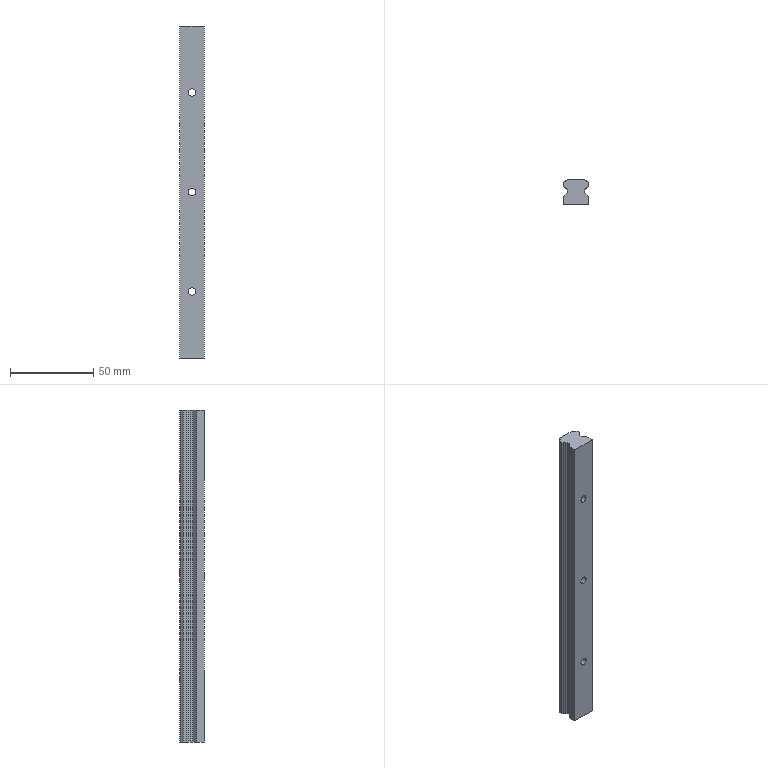Part | SolidWorks | features ICE 15, Chamfer 3, Extrusion 3, Fillet 3, MirrorPattern 3, MirrorSolid 3, RevCut 2, DeleteBody 1, Dome 1, LPattern 1 | 1 solid | 41 faces | box 15 x 15 x 200 mm | volume 39273 mm3 | plane 23 | cylinder 18 | commonest cylinder face diameters 1.459 x6 4.5 x6 7.5 x6
STEP:
#1=CARTESIAN_POINT('',(0.,5.3,-57.75));
#2=VERTEX_POINT('',#1);
#3=CARTESIAN_POINT('',(0.,5.3,-62.25));
#4=VERTEX_POINT('',#3);
#5=CARTESIAN_POINT('',(0.,5.3,-60.));
#6=DIRECTION('',(0.,-1.,0.));
#7=DIRECTION('',(0.,0.,-1.));
#8=AXIS2_PLACEMENT_3D('',#5,#6,#7);
#9=CIRCLE('',#8,2.25);
#10=EDGE_CURVE('',#2,#4,#9,.T.);
#11=ORIENTED_EDGE('',*,*,#10,.F.);
#12=CARTESIAN_POINT('',(0.,-4.4,-57.75));
#13=VERTEX_POINT('',#12);
#14=CARTESIAN_POINT('',(0.,-4.4,-57.75));
#15=DIRECTION('',(0.,-1.,0.));
#16=VECTOR('',#15,1000.);
#17=LINE('',#14,#16);
#18=EDGE_CURVE('',#2,#13,#17,.T.);
#19=ORIENTED_EDGE('',*,*,#18,.T.);
#20=CARTESIAN_POINT('',(0.,-4.4,-62.25));
#21=VERTEX_POINT('',#20);
#22=CARTESIAN_POINT('',(0.,-4.4,-60.));
#23=DIRECTION('',(0.,-1.,0.));
#24=DIRECTION('',(0.,0.,-1.));
#25=AXIS2_PLACEMENT_3D('',#22,#23,#24);
#26=CIRCLE('',#25,2.25);
#27=EDGE_CURVE('',#13,#21,#26,.T.);
#28=ORIENTED_EDGE('',*,*,#27,.T.);
#29=CARTESIAN_POINT('',(0.,-4.4,-62.25));
#30=DIRECTION('',(0.,-1.,0.));
#31=VECTOR('',#30,1000.);
#32=LINE('',#29,#31);
#33=EDGE_CURVE('',#4,#21,#32,.T.);
#34=ORIENTED_EDGE('',*,*,#33,.F.);
#35=EDGE_LOOP('',(#11,#19,#28,#34));
#36=FACE_OUTER_BOUND('',#35,.T.);
#37=CARTESIAN_POINT('',(0.,-4.4,-60.));
#38=DIRECTION('',(0.,-1.,0.));
#39=DIRECTION('',(0.,0.,-1.));
#40=AXIS2_PLACEMENT_3D('',#37,#38,#39);
#41=CYLINDRICAL_SURFACE('',#40,2.25);
#42=ADVANCED_FACE('',(#36),#41,.F.);
#43=CARTESIAN_POINT('',(0.,10.6,-56.25));
#44=VERTEX_POINT('',#43);
#45=CARTESIAN_POINT('',(0.,10.6,-63.75));
#46=VERTEX_POINT('',#45);
#47=CARTESIAN_POINT('',(0.,10.6,-60.));
#48=DIRECTION('',(0.,-1.,0.));
#49=DIRECTION('',(0.,0.,-1.));
#50=AXIS2_PLACEMENT_3D('',#47,#48,#49);
#51=CIRCLE('',#50,3.75);
#52=EDGE_CURVE('',#44,#46,#51,.T.);
#53=ORIENTED_EDGE('',*,*,#52,.F.);
#54=CARTESIAN_POINT('',(0.,5.3,-56.25));
#55=VERTEX_POINT('',#54);
#56=CARTESIAN_POINT('',(0.,-4.4,-56.25));
#57=DIRECTION('',(0.,-1.,0.));
#58=VECTOR('',#57,1000.);
#59=LINE('',#56,#58);
#60=EDGE_CURVE('',#44,#55,#59,.T.);
#61=ORIENTED_EDGE('',*,*,#60,.T.);
#62=CARTESIAN_POINT('',(0.,5.3,-63.75));
#63=VERTEX_POINT('',#62);
#64=CARTESIAN_POINT('',(0.,5.3,-60.));
#65=DIRECTION('',(0.,-1.,0.));
#66=DIRECTION('',(0.,0.,-1.));
#67=AXIS2_PLACEMENT_3D('',#64,#65,#66);
#68=CIRCLE('',#67,3.75);
#69=EDGE_CURVE('',#55,#63,#68,.T.);
#70=ORIENTED_EDGE('',*,*,#69,.T.);
#71=CARTESIAN_POINT('',(0.,-4.4,-63.75));
#72=DIRECTION('',(0.,-1.,0.));
#73=VECTOR('',#72,1000.);
#74=LINE('',#71,#73);
#75=EDGE_CURVE('',#46,#63,#74,.T.);
#76=ORIENTED_EDGE('',*,*,#75,.F.);
#77=EDGE_LOOP('',(#53,#61,#70,#76));
#78=FACE_OUTER_BOUND('',#77,.T.);
#79=CARTESIAN_POINT('',(0.,-4.4,-60.));
#80=DIRECTION('',(0.,-1.,0.));
#81=DIRECTION('',(0.,0.,-1.));
#82=AXIS2_PLACEMENT_3D('',#79,#80,#81);
#83=CYLINDRICAL_SURFACE('',#82,3.75);
#84=ADVANCED_FACE('',(#78),#83,.F.);
#85=CARTESIAN_POINT('',(0.,5.3,2.25));
#86=VERTEX_POINT('',#85);
#87=CARTESIAN_POINT('',(0.,5.3,-2.25));
#88=VERTEX_POINT('',#87);
#89=CARTESIAN_POINT('',(0.,5.3,0.));
#90=DIRECTION('',(0.,-1.,0.));
#91=DIRECTION('',(0.,0.,-1.));
#92=AXIS2_PLACEMENT_3D('',#89,#90,#91);
#93=CIRCLE('',#92,2.25);
#94=EDGE_CURVE('',#86,#88,#93,.T.);
#95=ORIENTED_EDGE('',*,*,#94,.F.);
#96=CARTESIAN_POINT('',(0.,-4.4,2.25));
#97=VERTEX_POINT('',#96);
#98=CARTESIAN_POINT('',(0.,-4.4,2.25));
#99=DIRECTION('',(0.,-1.,0.));
#100=VECTOR('',#99,1000.);
#101=LINE('',#98,#100);
#102=EDGE_CURVE('',#86,#97,#101,.T.);
#103=ORIENTED_EDGE('',*,*,#102,.T.);
#104=CARTESIAN_POINT('',(0.,-4.4,-2.25));
#105=VERTEX_POINT('',#104);
#106=CARTESIAN_POINT('',(0.,-4.4,0.));
#107=DIRECTION('',(0.,-1.,0.));
#108=DIRECTION('',(0.,0.,-1.));
#109=AXIS2_PLACEMENT_3D('',#106,#107,#108);
#110=CIRCLE('',#109,2.25);
#111=EDGE_CURVE('',#97,#105,#110,.T.);
#112=ORIENTED_EDGE('',*,*,#111,.T.);
#113=CARTESIAN_POINT('',(0.,-4.4,-2.25));
#114=DIRECTION('',(0.,-1.,0.));
#115=VECTOR('',#114,1000.);
#116=LINE('',#113,#115);
#117=EDGE_CURVE('',#88,#105,#116,.T.);
#118=ORIENTED_EDGE('',*,*,#117,.F.);
#119=EDGE_LOOP('',(#95,#103,#112,#118));
#120=FACE_OUTER_BOUND('',#119,.T.);
#121=CARTESIAN_POINT('',(0.,-4.4,0.));
#122=DIRECTION('',(0.,-1.,0.));
#123=DIRECTION('',(0.,0.,-1.));
#124=AXIS2_PLACEMENT_3D('',#121,#122,#123);
#125=CYLINDRICAL_SURFACE('',#124,2.25);
#126=ADVANCED_FACE('',(#120),#125,.F.);
#127=CARTESIAN_POINT('',(0.,10.6,3.75));
#128=VERTEX_POINT('',#127);
#129=CARTESIAN_POINT('',(0.,10.6,-3.75));
#130=VERTEX_POINT('',#129);
#131=CARTESIAN_POINT('',(0.,10.6,0.));
#132=DIRECTION('',(0.,-1.,0.));
#133=DIRECTION('',(0.,0.,-1.));
#134=AXIS2_PLACEMENT_3D('',#131,#132,#133);
#135=CIRCLE('',#134,3.75);
#136=EDGE_CURVE('',#128,#130,#135,.T.);
#137=ORIENTED_EDGE('',*,*,#136,.F.);
#138=CARTESIAN_POINT('',(0.,5.3,3.75));
#139=VERTEX_POINT('',#138);
#140=CARTESIAN_POINT('',(0.,-4.4,3.75));
#141=DIRECTION('',(0.,-1.,0.));
#142=VECTOR('',#141,1000.);
#143=LINE('',#140,#142);
#144=EDGE_CURVE('',#128,#139,#143,.T.);
#145=ORIENTED_EDGE('',*,*,#144,.T.);
#146=CARTESIAN_POINT('',(0.,5.3,-3.75));
#147=VERTEX_POINT('',#146);
#148=CARTESIAN_POINT('',(0.,5.3,0.));
#149=DIRECTION('',(0.,-1.,0.));
#150=DIRECTION('',(0.,0.,-1.));
#151=AXIS2_PLACEMENT_3D('',#148,#149,#150);
#152=CIRCLE('',#151,3.75);
#153=EDGE_CURVE('',#139,#147,#152,.T.);
#154=ORIENTED_EDGE('',*,*,#153,.T.);
#155=CARTESIAN_POINT('',(0.,-4.4,-3.75));
#156=DIRECTION('',(0.,-1.,0.));
#157=VECTOR('',#156,1000.);
#158=LINE('',#155,#157);
#159=EDGE_CURVE('',#130,#147,#158,.T.);
#160=ORIENTED_EDGE('',*,*,#159,.F.);
#161=EDGE_LOOP('',(#137,#145,#154,#160));
#162=FACE_OUTER_BOUND('',#161,.T.);
#163=CARTESIAN_POINT('',(0.,-4.4,0.));
#164=DIRECTION('',(0.,-1.,0.));
#165=DIRECTION('',(0.,0.,-1.));
#166=AXIS2_PLACEMENT_3D('',#163,#164,#165);
#167=CYLINDRICAL_SURFACE('',#166,3.75);
#168=ADVANCED_FACE('',(#162),#167,.F.);
#169=CARTESIAN_POINT('',(0.,5.3,62.25));
#170=VERTEX_POINT('',#169);
#171=CARTESIAN_POINT('',(0.,5.3,57.75));
#172=VERTEX_POINT('',#171);
#173=CARTESIAN_POINT('',(0.,5.3,60.));
#174=DIRECTION('',(0.,-1.,0.));
#175=DIRECTION('',(0.,0.,-1.));
#176=AXIS2_PLACEMENT_3D('',#173,#174,#175);
#177=CIRCLE('',#176,2.25);
#178=EDGE_CURVE('',#170,#172,#177,.T.);
#179=ORIENTED_EDGE('',*,*,#178,.F.);
#180=CARTESIAN_POINT('',(0.,-4.4,62.25));
#181=VERTEX_POINT('',#180);
#182=CARTESIAN_POINT('',(0.,-4.4,62.25));
#183=DIRECTION('',(0.,-1.,0.));
#184=VECTOR('',#183,1000.);
#185=LINE('',#182,#184);
#186=EDGE_CURVE('',#170,#181,#185,.T.);
#187=ORIENTED_EDGE('',*,*,#186,.T.);
#188=CARTESIAN_POINT('',(0.,-4.4,57.75));
#189=VERTEX_POINT('',#188);
#190=CARTESIAN_POINT('',(0.,-4.4,60.));
#191=DIRECTION('',(0.,-1.,0.));
#192=DIRECTION('',(0.,0.,-1.));
#193=AXIS2_PLACEMENT_3D('',#190,#191,#192);
#194=CIRCLE('',#193,2.25);
#195=EDGE_CURVE('',#181,#189,#194,.T.);
#196=ORIENTED_EDGE('',*,*,#195,.T.);
#197=CARTESIAN_POINT('',(0.,-4.4,57.75));
#198=DIRECTION('',(0.,-1.,0.));
#199=VECTOR('',#198,1000.);
#200=LINE('',#197,#199);
#201=EDGE_CURVE('',#172,#189,#200,.T.);
#202=ORIENTED_EDGE('',*,*,#201,.F.);
#203=EDGE_LOOP('',(#179,#187,#196,#202));
#204=FACE_OUTER_BOUND('',#203,.T.);
#205=CARTESIAN_POINT('',(0.,-4.4,60.));
#206=DIRECTION('',(0.,-1.,0.));
#207=DIRECTION('',(0.,0.,-1.));
#208=AXIS2_PLACEMENT_3D('',#205,#206,#207);
#209=CYLINDRICAL_SURFACE('',#208,2.25);
#210=ADVANCED_FACE('',(#204),#209,.F.);
#211=CARTESIAN_POINT('',(0.,10.6,63.75));
#212=VERTEX_POINT('',#211);
#213=CARTESIAN_POINT('',(0.,10.6,56.25));
#214=VERTEX_POINT('',#213);
#215=CARTESIAN_POINT('',(0.,10.6,60.));
#216=DIRECTION('',(0.,-1.,0.));
#217=DIRECTION('',(0.,0.,-1.));
#218=AXIS2_PLACEMENT_3D('',#215,#216,#217);
#219=CIRCLE('',#218,3.75);
#220=EDGE_CURVE('',#212,#214,#219,.T.);
#221=ORIENTED_EDGE('',*,*,#220,.F.);
#222=CARTESIAN_POINT('',(0.,5.3,63.75));
#223=VERTEX_POINT('',#222);
#224=CARTESIAN_POINT('',(0.,-4.4,63.75));
#225=DIRECTION('',(0.,-1.,0.));
#226=VECTOR('',#225,1000.);
#227=LINE('',#224,#226);
#228=EDGE_CURVE('',#212,#223,#227,.T.);
#229=ORIENTED_EDGE('',*,*,#228,.T.);
#230=CARTESIAN_POINT('',(0.,5.3,56.25));
#231=VERTEX_POINT('',#230);
#232=CARTESIAN_POINT('',(0.,5.3,60.));
#233=DIRECTION('',(0.,-1.,0.));
#234=DIRECTION('',(0.,0.,-1.));
#235=AXIS2_PLACEMENT_3D('',#232,#233,#234);
#236=CIRCLE('',#235,3.75);
#237=EDGE_CURVE('',#223,#231,#236,.T.);
#238=ORIENTED_EDGE('',*,*,#237,.T.);
#239=CARTESIAN_POINT('',(0.,-4.4,56.25));
#240=DIRECTION('',(0.,-1.,0.));
#241=VECTOR('',#240,1000.);
#242=LINE('',#239,#241);
#243=EDGE_CURVE('',#214,#231,#242,.T.);
#244=ORIENTED_EDGE('',*,*,#243,.F.);
#245=EDGE_LOOP('',(#221,#229,#238,#244));
#246=FACE_OUTER_BOUND('',#245,.T.);
#247=CARTESIAN_POINT('',(0.,-4.4,60.));
#248=DIRECTION('',(0.,-1.,0.));
#249=DIRECTION('',(0.,0.,-1.));
#250=AXIS2_PLACEMENT_3D('',#247,#248,#249);
#251=CYLINDRICAL_SURFACE('',#250,3.75);
#252=ADVANCED_FACE('',(#246),#251,.F.);
#253=CARTESIAN_POINT('',(-6.016,9.858,-100.));
#254=VERTEX_POINT('',#253);
#255=CARTESIAN_POINT('',(-6.016,9.846,-100.));
#256=VERTEX_POINT('',#255);
#257=CARTESIAN_POINT('',(-6.746,9.846,-100.));
#258=DIRECTION('',(0.,0.,-1.));
#259=DIRECTION('',(1.,0.,0.));
#260=AXIS2_PLACEMENT_3D('',#257,#258,#259);
#261=CIRCLE('',#260,0.7296);
#262=EDGE_CURVE('',#254,#256,#261,.T.);
#263=ORIENTED_EDGE('',*,*,#262,.T.);
#264=CARTESIAN_POINT('',(-6.016,9.846,100.));
#265=VERTEX_POINT('',#264);
#266=CARTESIAN_POINT('',(-6.016,9.846,-100.));
#267=DIRECTION('',(0.,0.,1.));
#268=VECTOR('',#267,1000.);
#269=LINE('',#266,#268);
#270=EDGE_CURVE('',#256,#265,#269,.T.);
#271=ORIENTED_EDGE('',*,*,#270,.T.);
#272=CARTESIAN_POINT('',(-6.016,9.858,100.));
#273=VERTEX_POINT('',#272);
#274=CARTESIAN_POINT('',(-6.746,9.846,100.));
#275=DIRECTION('',(0.,0.,-1.));
#276=DIRECTION('',(1.,0.,0.));
#277=AXIS2_PLACEMENT_3D('',#274,#275,#276);
#278=CIRCLE('',#277,0.7296);
#279=EDGE_CURVE('',#273,#265,#278,.T.);
#280=ORIENTED_EDGE('',*,*,#279,.F.);
#281=CARTESIAN_POINT('',(-6.016,9.858,-100.));
#282=DIRECTION('',(0.,0.,1.));
#283=VECTOR('',#282,1000.);
#284=LINE('',#281,#283);
#285=EDGE_CURVE('',#254,#273,#284,.T.);
#286=ORIENTED_EDGE('',*,*,#285,.F.);
#287=EDGE_LOOP('',(#263,#271,#280,#286));
#288=FACE_OUTER_BOUND('',#287,.T.);
#289=CARTESIAN_POINT('',(-6.746,9.846,-100.));
#290=DIRECTION('',(0.,0.,1.));
#291=DIRECTION('',(1.,0.,0.));
#292=AXIS2_PLACEMENT_3D('',#289,#290,#291);
#293=CYLINDRICAL_SURFACE('',#292,0.7296);
#294=ADVANCED_FACE('',(#288),#293,.F.);
#295=CARTESIAN_POINT('',(-6.758,5.724,-100.));
#296=VERTEX_POINT('',#295);
#297=CARTESIAN_POINT('',(-6.016,4.994,-100.));
#298=VERTEX_POINT('',#297);
#299=CARTESIAN_POINT('',(-6.746,4.994,-100.));
#300=DIRECTION('',(0.,0.,-1.));
#301=DIRECTION('',(1.,0.,0.));
#302=AXIS2_PLACEMENT_3D('',#299,#300,#301);
#303=CIRCLE('',#302,0.7296);
#304=EDGE_CURVE('',#296,#298,#303,.T.);
#305=ORIENTED_EDGE('',*,*,#304,.T.);
#306=CARTESIAN_POINT('',(-6.016,4.994,100.));
#307=VERTEX_POINT('',#306);
#308=CARTESIAN_POINT('',(-6.016,4.994,-100.));
#309=DIRECTION('',(0.,0.,1.));
#310=VECTOR('',#309,1000.);
#311=LINE('',#308,#310);
#312=EDGE_CURVE('',#298,#307,#311,.T.);
#313=ORIENTED_EDGE('',*,*,#312,.T.);
#314=CARTESIAN_POINT('',(-6.758,5.724,100.));
#315=VERTEX_POINT('',#314);
#316=CARTESIAN_POINT('',(-6.746,4.994,100.));
#317=DIRECTION('',(0.,0.,-1.));
#318=DIRECTION('',(1.,0.,0.));
#319=AXIS2_PLACEMENT_3D('',#316,#317,#318);
#320=CIRCLE('',#319,0.7296);
#321=EDGE_CURVE('',#315,#307,#320,.T.);
#322=ORIENTED_EDGE('',*,*,#321,.F.);
#323=CARTESIAN_POINT('',(-6.758,5.724,-100.));
#324=DIRECTION('',(0.,0.,1.));
#325=VECTOR('',#324,1000.);
#326=LINE('',#323,#325);
#327=EDGE_CURVE('',#296,#315,#326,.T.);
#328=ORIENTED_EDGE('',*,*,#327,.F.);
#329=EDGE_LOOP('',(#305,#313,#322,#328));
#330=FACE_OUTER_BOUND('',#329,.T.);
#331=CARTESIAN_POINT('',(-6.746,4.994,-100.));
#332=DIRECTION('',(0.,0.,1.));
#333=DIRECTION('',(1.,0.,0.));
#334=AXIS2_PLACEMENT_3D('',#331,#332,#333);
#335=CYLINDRICAL_SURFACE('',#334,0.7296);
#336=ADVANCED_FACE('',(#330),#335,.F.);
#337=CARTESIAN_POINT('',(5.274,10.6,-100.));
#338=VERTEX_POINT('',#337);
#339=CARTESIAN_POINT('',(5.274,10.6,100.));
#340=VERTEX_POINT('',#339);
#341=CARTESIAN_POINT('',(5.274,10.6,-100.));
#342=DIRECTION('',(0.,0.,1.));
#343=VECTOR('',#342,1000.);
#344=LINE('',#341,#343);
#345=EDGE_CURVE('',#338,#340,#344,.T.);
#346=ORIENTED_EDGE('',*,*,#345,.T.);
#347=CARTESIAN_POINT('',(6.016,9.858,100.));
#348=VERTEX_POINT('',#347);
#349=CARTESIAN_POINT('',(6.016,9.858,100.));
#350=DIRECTION('',(-0.7071,0.7071,0.));
#351=VECTOR('',#350,1000.);
#352=LINE('',#349,#351);
#353=EDGE_CURVE('',#348,#340,#352,.T.);
#354=ORIENTED_EDGE('',*,*,#353,.F.);
#355=CARTESIAN_POINT('',(6.016,9.858,-100.));
#356=VERTEX_POINT('',#355);
#357=CARTESIAN_POINT('',(6.016,9.858,-100.));
#358=DIRECTION('',(0.,0.,1.));
#359=VECTOR('',#358,1000.);
#360=LINE('',#357,#359);
#361=EDGE_CURVE('',#356,#348,#360,.T.);
#362=ORIENTED_EDGE('',*,*,#361,.F.);
#363=CARTESIAN_POINT('',(6.016,9.858,-100.));
#364=DIRECTION('',(-0.7071,0.7071,0.));
#365=VECTOR('',#364,1000.);
#366=LINE('',#363,#365);
#367=EDGE_CURVE('',#356,#338,#366,.T.);
#368=ORIENTED_EDGE('',*,*,#367,.T.);
#369=EDGE_LOOP('',(#346,#354,#362,#368));
#370=FACE_OUTER_BOUND('',#369,.T.);
#371=CARTESIAN_POINT('',(6.016,9.858,-100.));
#372=DIRECTION('',(0.7071,0.7071,0.));
#373=DIRECTION('',(-0.7071,0.7071,0.));
#374=AXIS2_PLACEMENT_3D('',#371,#372,#373);
#375=PLANE('',#374);
#376=ADVANCED_FACE('',(#370),#375,.T.);
#377=ORIENTED_EDGE('',*,*,#361,.T.);
#378=CARTESIAN_POINT('',(6.758,9.116,100.));
#379=VERTEX_POINT('',#378);
#380=CARTESIAN_POINT('',(6.746,9.846,100.));
#381=DIRECTION('',(0.,0.,-1.));
#382=DIRECTION('',(1.,0.,0.));
#383=AXIS2_PLACEMENT_3D('',#380,#381,#382);
#384=CIRCLE('',#383,0.7296);
#385=EDGE_CURVE('',#379,#348,#384,.T.);
#386=ORIENTED_EDGE('',*,*,#385,.F.);
#387=CARTESIAN_POINT('',(6.758,9.116,-100.));
#388=VERTEX_POINT('',#387);
#389=CARTESIAN_POINT('',(6.758,9.116,-100.));
#390=DIRECTION('',(0.,0.,1.));
#391=VECTOR('',#390,1000.);
#392=LINE('',#389,#391);
#393=EDGE_CURVE('',#388,#379,#392,.T.);
#394=ORIENTED_EDGE('',*,*,#393,.F.);
#395=CARTESIAN_POINT('',(6.746,9.846,-100.));
#396=DIRECTION('',(0.,0.,-1.));
#397=DIRECTION('',(1.,0.,0.));
#398=AXIS2_PLACEMENT_3D('',#395,#396,#397);
#399=CIRCLE('',#398,0.7296);
#400=EDGE_CURVE('',#388,#356,#399,.T.);
#401=ORIENTED_EDGE('',*,*,#400,.T.);
#402=EDGE_LOOP('',(#377,#386,#394,#401));
#403=FACE_OUTER_BOUND('',#402,.T.);
#404=CARTESIAN_POINT('',(6.746,9.846,-100.));
#405=DIRECTION('',(0.,0.,1.));
#406=DIRECTION('',(1.,0.,0.));
#407=AXIS2_PLACEMENT_3D('',#404,#405,#406);
#408=CYLINDRICAL_SURFACE('',#407,0.7296);
#409=ADVANCED_FACE('',(#403),#408,.F.);
#410=ORIENTED_EDGE('',*,*,#393,.T.);
#411=CARTESIAN_POINT('',(7.5,8.374,100.));
#412=VERTEX_POINT('',#411);
#413=CARTESIAN_POINT('',(7.5,8.374,100.));
#414=DIRECTION('',(-0.7071,0.7071,0.));
#415=VECTOR('',#414,1000.);
#416=LINE('',#413,#415);
#417=EDGE_CURVE('',#412,#379,#416,.T.);
#418=ORIENTED_EDGE('',*,*,#417,.F.);
#419=CARTESIAN_POINT('',(7.5,8.374,-100.));
#420=VERTEX_POINT('',#419);
#421=CARTESIAN_POINT('',(7.5,8.374,-100.));
#422=DIRECTION('',(0.,0.,1.));
#423=VECTOR('',#422,1000.);
#424=LINE('',#421,#423);
#425=EDGE_CURVE('',#420,#412,#424,.T.);
#426=ORIENTED_EDGE('',*,*,#425,.F.);
#427=CARTESIAN_POINT('',(7.5,8.374,-100.));
#428=DIRECTION('',(-0.7071,0.7071,0.));
#429=VECTOR('',#428,1000.);
#430=LINE('',#427,#429);
#431=EDGE_CURVE('',#420,#388,#430,.T.);
#432=ORIENTED_EDGE('',*,*,#431,.T.);
#433=EDGE_LOOP('',(#410,#418,#426,#432));
#434=FACE_OUTER_BOUND('',#433,.T.);
#435=CARTESIAN_POINT('',(7.5,8.374,-100.));
#436=DIRECTION('',(0.7071,0.7071,0.));
#437=DIRECTION('',(-0.7071,0.7071,0.));
#438=AXIS2_PLACEMENT_3D('',#435,#436,#437);
#439=PLANE('',#438);
#440=ADVANCED_FACE('',(#434),#439,.T.);
#441=ORIENTED_EDGE('',*,*,#425,.T.);
#442=CARTESIAN_POINT('',(7.5,6.466,100.));
#443=VERTEX_POINT('',#442);
#444=CARTESIAN_POINT('',(7.5,6.466,100.));
#445=DIRECTION('',(0.,1.,0.));
#446=VECTOR('',#445,1000.);
#447=LINE('',#444,#446);
#448=EDGE_CURVE('',#443,#412,#447,.T.);
#449=ORIENTED_EDGE('',*,*,#448,.F.);
#450=CARTESIAN_POINT('',(7.5,6.466,-100.));
#451=VERTEX_POINT('',#450);
#452=CARTESIAN_POINT('',(7.5,6.466,-100.));
#453=DIRECTION('',(0.,0.,1.));
#454=VECTOR('',#453,1000.);
#455=LINE('',#452,#454);
#456=EDGE_CURVE('',#451,#443,#455,.T.);
#457=ORIENTED_EDGE('',*,*,#456,.F.);
#458=CARTESIAN_POINT('',(7.5,6.466,-100.));
#459=DIRECTION('',(0.,1.,0.));
#460=VECTOR('',#459,1000.);
#461=LINE('',#458,#460);
#462=EDGE_CURVE('',#451,#420,#461,.T.);
#463=ORIENTED_EDGE('',*,*,#462,.T.);
#464=EDGE_LOOP('',(#441,#449,#457,#463));
#465=FACE_OUTER_BOUND('',#464,.T.);
#466=CARTESIAN_POINT('',(7.5,6.466,-100.));
#467=DIRECTION('',(1.,0.,0.));
#468=DIRECTION('',(0.,0.,-1.));
#469=AXIS2_PLACEMENT_3D('',#466,#467,#468);
#470=PLANE('',#469);
#471=ADVANCED_FACE('',(#465),#470,.T.);
#472=ORIENTED_EDGE('',*,*,#456,.T.);
#473=CARTESIAN_POINT('',(6.758,5.724,100.));
#474=VERTEX_POINT('',#473);
#475=CARTESIAN_POINT('',(6.758,5.724,100.));
#476=DIRECTION('',(0.7071,0.7071,0.));
#477=VECTOR('',#476,1000.);
#478=LINE('',#475,#477);
#479=EDGE_CURVE('',#474,#443,#478,.T.);
#480=ORIENTED_EDGE('',*,*,#479,.F.);
#481=CARTESIAN_POINT('',(6.758,5.724,-100.));
#482=VERTEX_POINT('',#481);
#483=CARTESIAN_POINT('',(6.758,5.724,-100.));
#484=DIRECTION('',(0.,0.,1.));
#485=VECTOR('',#484,1000.);
#486=LINE('',#483,#485);
#487=EDGE_CURVE('',#482,#474,#486,.T.);
#488=ORIENTED_EDGE('',*,*,#487,.F.);
#489=CARTESIAN_POINT('',(6.758,5.724,-100.));
#490=DIRECTION('',(0.7071,0.7071,0.));
#491=VECTOR('',#490,1000.);
#492=LINE('',#489,#491);
#493=EDGE_CURVE('',#482,#451,#492,.T.);
#494=ORIENTED_EDGE('',*,*,#493,.T.);
#495=EDGE_LOOP('',(#472,#480,#488,#494));
#496=FACE_OUTER_BOUND('',#495,.T.);
#497=CARTESIAN_POINT('',(6.758,5.724,-100.));
#498=DIRECTION('',(0.7071,-0.7071,0.));
#499=DIRECTION('',(0.7071,0.7071,0.));
#500=AXIS2_PLACEMENT_3D('',#497,#498,#499);
#501=PLANE('',#500);
#502=ADVANCED_FACE('',(#496),#501,.T.);
#503=ORIENTED_EDGE('',*,*,#487,.T.);
#504=CARTESIAN_POINT('',(6.016,4.982,100.));
#505=VERTEX_POINT('',#504);
#506=CARTESIAN_POINT('',(6.746,4.994,100.));
#507=DIRECTION('',(0.,0.,-1.));
#508=DIRECTION('',(1.,0.,0.));
#509=AXIS2_PLACEMENT_3D('',#506,#507,#508);
#510=CIRCLE('',#509,0.7296);
#511=EDGE_CURVE('',#505,#474,#510,.T.);
#512=ORIENTED_EDGE('',*,*,#511,.F.);
#513=CARTESIAN_POINT('',(6.016,4.982,-100.));
#514=VERTEX_POINT('',#513);
#515=CARTESIAN_POINT('',(6.016,4.982,-100.));
#516=DIRECTION('',(0.,0.,1.));
#517=VECTOR('',#516,1000.);
#518=LINE('',#515,#517);
#519=EDGE_CURVE('',#514,#505,#518,.T.);
#520=ORIENTED_EDGE('',*,*,#519,.F.);
#521=CARTESIAN_POINT('',(6.746,4.994,-100.));
#522=DIRECTION('',(0.,0.,-1.));
#523=DIRECTION('',(1.,0.,0.));
#524=AXIS2_PLACEMENT_3D('',#521,#522,#523);
#525=CIRCLE('',#524,0.7296);
#526=EDGE_CURVE('',#514,#482,#525,.T.);
#527=ORIENTED_EDGE('',*,*,#526,.T.);
#528=EDGE_LOOP('',(#503,#512,#520,#527));
#529=FACE_OUTER_BOUND('',#528,.T.);
#530=CARTESIAN_POINT('',(6.746,4.994,-100.));
#531=DIRECTION('',(0.,0.,1.));
#532=DIRECTION('',(1.,0.,0.));
#533=AXIS2_PLACEMENT_3D('',#530,#531,#532);
#534=CYLINDRICAL_SURFACE('',#533,0.7296);
#535=ADVANCED_FACE('',(#529),#534,.F.);
#536=ORIENTED_EDGE('',*,*,#519,.T.);
#537=CARTESIAN_POINT('',(5.274,4.24,100.));
#538=VERTEX_POINT('',#537);
#539=CARTESIAN_POINT('',(5.274,4.24,100.));
#540=DIRECTION('',(0.7071,0.7071,0.));
#541=VECTOR('',#540,1000.);
#542=LINE('',#539,#541);
#543=EDGE_CURVE('',#538,#505,#542,.T.);
#544=ORIENTED_EDGE('',*,*,#543,.F.);
#545=CARTESIAN_POINT('',(5.274,4.24,-100.));
#546=VERTEX_POINT('',#545);
#547=CARTESIAN_POINT('',(5.274,4.24,-100.));
#548=DIRECTION('',(0.,0.,1.));
#549=VECTOR('',#548,1000.);
#550=LINE('',#547,#549);
#551=EDGE_CURVE('',#546,#538,#550,.T.);
#552=ORIENTED_EDGE('',*,*,#551,.F.);
#553=CARTESIAN_POINT('',(5.274,4.24,-100.));
#554=DIRECTION('',(0.7071,0.7071,0.));
#555=VECTOR('',#554,1000.);
#556=LINE('',#553,#555);
#557=EDGE_CURVE('',#546,#514,#556,.T.);
#558=ORIENTED_EDGE('',*,*,#557,.T.);
#559=EDGE_LOOP('',(#536,#544,#552,#558));
#560=FACE_OUTER_BOUND('',#559,.T.);
#561=CARTESIAN_POINT('',(5.274,4.24,-100.));
#562=DIRECTION('',(0.7071,-0.7071,0.));
#563=DIRECTION('',(0.7071,0.7071,0.));
#564=AXIS2_PLACEMENT_3D('',#561,#562,#563);
#565=PLANE('',#564);
#566=ADVANCED_FACE('',(#560),#565,.T.);
#567=ORIENTED_EDGE('',*,*,#551,.T.);
#568=CARTESIAN_POINT('',(5.274,2.601,100.));
#569=VERTEX_POINT('',#568);
#570=CARTESIAN_POINT('',(5.274,2.601,100.));
#571=DIRECTION('',(0.,1.,0.));
#572=VECTOR('',#571,1000.);
#573=LINE('',#570,#572);
#574=EDGE_CURVE('',#569,#538,#573,.T.);
#575=ORIENTED_EDGE('',*,*,#574,.F.);
#576=CARTESIAN_POINT('',(5.274,2.601,-100.));
#577=VERTEX_POINT('',#576);
#578=CARTESIAN_POINT('',(5.274,2.601,-100.));
#579=DIRECTION('',(0.,0.,1.));
#580=VECTOR('',#579,1000.);
#581=LINE('',#578,#580);
#582=EDGE_CURVE('',#577,#569,#581,.T.);
#583=ORIENTED_EDGE('',*,*,#582,.F.);
#584=CARTESIAN_POINT('',(5.274,2.601,-100.));
#585=DIRECTION('',(0.,1.,0.));
#586=VECTOR('',#585,1000.);
#587=LINE('',#584,#586);
#588=EDGE_CURVE('',#577,#546,#587,.T.);
#589=ORIENTED_EDGE('',*,*,#588,.T.);
#590=EDGE_LOOP('',(#567,#575,#583,#589));
#591=FACE_OUTER_BOUND('',#590,.T.);
#592=CARTESIAN_POINT('',(5.274,2.601,-100.));
#593=DIRECTION('',(1.,0.,0.));
#594=DIRECTION('',(0.,1.,0.));
#595=AXIS2_PLACEMENT_3D('',#592,#593,#594);
#596=PLANE('',#595);
#597=ADVANCED_FACE('',(#591),#596,.T.);
#598=ORIENTED_EDGE('',*,*,#582,.T.);
#599=CARTESIAN_POINT('',(7.5,0.375,100.));
#600=VERTEX_POINT('',#599);
#601=CARTESIAN_POINT('',(7.5,0.375,100.));
#602=DIRECTION('',(-0.7071,0.7071,0.));
#603=VECTOR('',#602,1000.);
#604=LINE('',#601,#603);
#605=EDGE_CURVE('',#600,#569,#604,.T.);
#606=ORIENTED_EDGE('',*,*,#605,.F.);
#607=CARTESIAN_POINT('',(7.5,0.375,-100.));
#608=VERTEX_POINT('',#607);
#609=CARTESIAN_POINT('',(7.5,0.375,-100.));
#610=DIRECTION('',(0.,0.,1.));
#611=VECTOR('',#610,1000.);
#612=LINE('',#609,#611);
#613=EDGE_CURVE('',#608,#600,#612,.T.);
#614=ORIENTED_EDGE('',*,*,#613,.F.);
#615=CARTESIAN_POINT('',(7.5,0.375,-100.));
#616=DIRECTION('',(-0.7071,0.7071,0.));
#617=VECTOR('',#616,1000.);
#618=LINE('',#615,#617);
#619=EDGE_CURVE('',#608,#577,#618,.T.);
#620=ORIENTED_EDGE('',*,*,#619,.T.);
#621=EDGE_LOOP('',(#598,#606,#614,#620));
#622=FACE_OUTER_BOUND('',#621,.T.);
#623=CARTESIAN_POINT('',(7.5,0.375,-100.));
#624=DIRECTION('',(0.7071,0.7071,0.));
#625=DIRECTION('',(-0.7071,0.7071,0.));
#626=AXIS2_PLACEMENT_3D('',#623,#624,#625);
#627=PLANE('',#626);
#628=ADVANCED_FACE('',(#622),#627,.T.);
#629=ORIENTED_EDGE('',*,*,#613,.T.);
#630=CARTESIAN_POINT('',(7.5,-4.4,100.));
#631=VERTEX_POINT('',#630);
#632=CARTESIAN_POINT('',(7.5,-4.4,100.));
#633=DIRECTION('',(0.,1.,0.));
#634=VECTOR('',#633,1000.);
#635=LINE('',#632,#634);
#636=EDGE_CURVE('',#631,#600,#635,.T.);
#637=ORIENTED_EDGE('',*,*,#636,.F.);
#638=CARTESIAN_POINT('',(7.5,-4.4,-100.));
#639=VERTEX_POINT('',#638);
#640=CARTESIAN_POINT('',(7.5,-4.4,-100.));
#641=DIRECTION('',(0.,0.,1.));
#642=VECTOR('',#641,1000.);
#643=LINE('',#640,#642);
#644=EDGE_CURVE('',#639,#631,#643,.T.);
#645=ORIENTED_EDGE('',*,*,#644,.F.);
#646=CARTESIAN_POINT('',(7.5,-4.4,-100.));
#647=DIRECTION('',(0.,1.,0.));
#648=VECTOR('',#647,1000.);
#649=LINE('',#646,#648);
#650=EDGE_CURVE('',#639,#608,#649,.T.);
#651=ORIENTED_EDGE('',*,*,#650,.T.);
#652=EDGE_LOOP('',(#629,#637,#645,#651));
#653=FACE_OUTER_BOUND('',#652,.T.);
#654=CARTESIAN_POINT('',(7.5,-4.4,-100.));
#655=DIRECTION('',(1.,0.,0.));
#656=DIRECTION('',(0.,0.,-1.));
#657=AXIS2_PLACEMENT_3D('',#654,#655,#656);
#658=PLANE('',#657);
#659=ADVANCED_FACE('',(#653),#658,.T.);
#660=CARTESIAN_POINT('',(0.,-4.4,-60.));
#661=DIRECTION('',(0.,-1.,0.));
#662=DIRECTION('',(0.,0.,-1.));
#663=AXIS2_PLACEMENT_3D('',#660,#661,#662);
#664=CIRCLE('',#663,2.25);
#665=EDGE_CURVE('',#21,#13,#664,.T.);
#666=ORIENTED_EDGE('',*,*,#665,.F.);
#667=ORIENTED_EDGE('',*,*,#27,.F.);
#668=EDGE_LOOP('',(#666,#667));
#669=FACE_BOUND('',#668,.T.);
#670=CARTESIAN_POINT('',(0.,-4.4,0.));
#671=DIRECTION('',(0.,-1.,0.));
#672=DIRECTION('',(0.,0.,-1.));
#673=AXIS2_PLACEMENT_3D('',#670,#671,#672);
#674=CIRCLE('',#673,2.25);
#675=EDGE_CURVE('',#105,#97,#674,.T.);
#676=ORIENTED_EDGE('',*,*,#675,.F.);
#677=ORIENTED_EDGE('',*,*,#111,.F.);
#678=EDGE_LOOP('',(#676,#677));
#679=FACE_BOUND('',#678,.T.);
#680=CARTESIAN_POINT('',(0.,-4.4,60.));
#681=DIRECTION('',(0.,-1.,0.));
#682=DIRECTION('',(0.,0.,-1.));
#683=AXIS2_PLACEMENT_3D('',#680,#681,#682);
#684=CIRCLE('',#683,2.25);
#685=EDGE_CURVE('',#189,#181,#684,.T.);
#686=ORIENTED_EDGE('',*,*,#685,.F.);
#687=ORIENTED_EDGE('',*,*,#195,.F.);
#688=EDGE_LOOP('',(#686,#687));
#689=FACE_BOUND('',#688,.T.);
#690=ORIENTED_EDGE('',*,*,#644,.T.);
#691=CARTESIAN_POINT('',(-7.5,-4.4,100.));
#692=VERTEX_POINT('',#691);
#693=CARTESIAN_POINT('',(-7.5,-4.4,100.));
#694=DIRECTION('',(1.,0.,0.));
#695=VECTOR('',#694,1000.);
#696=LINE('',#693,#695);
#697=EDGE_CURVE('',#692,#631,#696,.T.);
#698=ORIENTED_EDGE('',*,*,#697,.F.);
#699=CARTESIAN_POINT('',(-7.5,-4.4,-100.));
#700=VERTEX_POINT('',#699);
#701=CARTESIAN_POINT('',(-7.5,-4.4,-100.));
#702=DIRECTION('',(0.,0.,1.));
#703=VECTOR('',#702,1000.);
#704=LINE('',#701,#703);
#705=EDGE_CURVE('',#700,#692,#704,.T.);
#706=ORIENTED_EDGE('',*,*,#705,.F.);
#707=CARTESIAN_POINT('',(-7.5,-4.4,-100.));
#708=DIRECTION('',(1.,0.,0.));
#709=VECTOR('',#708,1000.);
#710=LINE('',#707,#709);
#711=EDGE_CURVE('',#700,#639,#710,.T.);
#712=ORIENTED_EDGE('',*,*,#711,.T.);
#713=EDGE_LOOP('',(#690,#698,#706,#712));
#714=FACE_OUTER_BOUND('',#713,.T.);
#715=CARTESIAN_POINT('',(-7.5,-4.4,-100.));
#716=DIRECTION('',(0.,-1.,0.));
#717=DIRECTION('',(1.,0.,0.));
#718=AXIS2_PLACEMENT_3D('',#715,#716,#717);
#719=PLANE('',#718);
#720=ADVANCED_FACE('',(#669,#679,#689,#714),#719,.T.);
#721=ORIENTED_EDGE('',*,*,#705,.T.);
#722=CARTESIAN_POINT('',(-7.5,0.375,100.));
#723=VERTEX_POINT('',#722);
#724=CARTESIAN_POINT('',(-7.5,-4.4,100.));
#725=DIRECTION('',(0.,-1.,0.));
#726=VECTOR('',#725,1000.);
#727=LINE('',#724,#726);
#728=EDGE_CURVE('',#723,#692,#727,.T.);
#729=ORIENTED_EDGE('',*,*,#728,.F.);
#730=CARTESIAN_POINT('',(-7.5,0.375,-100.));
#731=VERTEX_POINT('',#730);
#732=CARTESIAN_POINT('',(-7.5,0.375,-100.));
#733=DIRECTION('',(0.,0.,1.));
#734=VECTOR('',#733,1000.);
#735=LINE('',#732,#734);
#736=EDGE_CURVE('',#731,#723,#735,.T.);
#737=ORIENTED_EDGE('',*,*,#736,.F.);
#738=CARTESIAN_POINT('',(-7.5,-4.4,-100.));
#739=DIRECTION('',(0.,-1.,0.));
#740=VECTOR('',#739,1000.);
#741=LINE('',#738,#740);
#742=EDGE_CURVE('',#731,#700,#741,.T.);
#743=ORIENTED_EDGE('',*,*,#742,.T.);
#744=EDGE_LOOP('',(#721,#729,#737,#743));
#745=FACE_OUTER_BOUND('',#744,.T.);
#746=CARTESIAN_POINT('',(-7.5,-4.4,-100.));
#747=DIRECTION('',(-1.,0.,0.));
#748=DIRECTION('',(0.,-1.,0.));
#749=AXIS2_PLACEMENT_3D('',#746,#747,#748);
#750=PLANE('',#749);
#751=ADVANCED_FACE('',(#745),#750,.T.);
#752=ORIENTED_EDGE('',*,*,#736,.T.);
#753=CARTESIAN_POINT('',(-5.274,2.601,100.));
#754=VERTEX_POINT('',#753);
#755=CARTESIAN_POINT('',(-7.5,0.375,100.));
#756=DIRECTION('',(-0.7071,-0.7071,0.));
#757=VECTOR('',#756,1000.);
#758=LINE('',#755,#757);
#759=EDGE_CURVE('',#754,#723,#758,.T.);
#760=ORIENTED_EDGE('',*,*,#759,.F.);
#761=CARTESIAN_POINT('',(-5.274,2.601,-100.));
#762=VERTEX_POINT('',#761);
#763=CARTESIAN_POINT('',(-5.274,2.601,-100.));
#764=DIRECTION('',(0.,0.,1.));
#765=VECTOR('',#764,1000.);
#766=LINE('',#763,#765);
#767=EDGE_CURVE('',#762,#754,#766,.T.);
#768=ORIENTED_EDGE('',*,*,#767,.F.);
#769=CARTESIAN_POINT('',(-7.5,0.375,-100.));
#770=DIRECTION('',(-0.7071,-0.7071,0.));
#771=VECTOR('',#770,1000.);
#772=LINE('',#769,#771);
#773=EDGE_CURVE('',#762,#731,#772,.T.);
#774=ORIENTED_EDGE('',*,*,#773,.T.);
#775=EDGE_LOOP('',(#752,#760,#768,#774));
#776=FACE_OUTER_BOUND('',#775,.T.);
#777=CARTESIAN_POINT('',(-7.5,0.375,-100.));
#778=DIRECTION('',(-0.7071,0.7071,0.));
#779=DIRECTION('',(-0.7071,-0.7071,0.));
#780=AXIS2_PLACEMENT_3D('',#777,#778,#779);
#781=PLANE('',#780);
#782=ADVANCED_FACE('',(#776),#781,.T.);
#783=ORIENTED_EDGE('',*,*,#767,.T.);
#784=CARTESIAN_POINT('',(-5.274,4.24,100.));
#785=VERTEX_POINT('',#784);
#786=CARTESIAN_POINT('',(-5.274,2.601,100.));
#787=DIRECTION('',(0.,-1.,0.));
#788=VECTOR('',#787,1000.);
#789=LINE('',#786,#788);
#790=EDGE_CURVE('',#785,#754,#789,.T.);
#791=ORIENTED_EDGE('',*,*,#790,.F.);
#792=CARTESIAN_POINT('',(-5.274,4.24,-100.));
#793=VERTEX_POINT('',#792);
#794=CARTESIAN_POINT('',(-5.274,4.24,-100.));
#795=DIRECTION('',(0.,0.,1.));
#796=VECTOR('',#795,1000.);
#797=LINE('',#794,#796);
#798=EDGE_CURVE('',#793,#785,#797,.T.);
#799=ORIENTED_EDGE('',*,*,#798,.F.);
#800=CARTESIAN_POINT('',(-5.274,2.601,-100.));
#801=DIRECTION('',(0.,-1.,0.));
#802=VECTOR('',#801,1000.);
#803=LINE('',#800,#802);
#804=EDGE_CURVE('',#793,#762,#803,.T.);
#805=ORIENTED_EDGE('',*,*,#804,.T.);
#806=EDGE_LOOP('',(#783,#791,#799,#805));
#807=FACE_OUTER_BOUND('',#806,.T.);
#808=CARTESIAN_POINT('',(-5.274,2.601,-100.));
#809=DIRECTION('',(-1.,0.,0.));
#810=DIRECTION('',(0.,-1.,0.));
#811=AXIS2_PLACEMENT_3D('',#808,#809,#810);
#812=PLANE('',#811);
#813=ADVANCED_FACE('',(#807),#812,.T.);
#814=ORIENTED_EDGE('',*,*,#798,.T.);
#815=CARTESIAN_POINT('',(-6.016,4.982,100.));
#816=VERTEX_POINT('',#815);
#817=CARTESIAN_POINT('',(-5.274,4.24,100.));
#818=DIRECTION('',(0.7071,-0.7071,0.));
#819=VECTOR('',#818,1000.);
#820=LINE('',#817,#819);
#821=EDGE_CURVE('',#816,#785,#820,.T.);
#822=ORIENTED_EDGE('',*,*,#821,.F.);
#823=CARTESIAN_POINT('',(-6.016,4.982,-100.));
#824=VERTEX_POINT('',#823);
#825=CARTESIAN_POINT('',(-6.016,4.982,-100.));
#826=DIRECTION('',(0.,0.,1.));
#827=VECTOR('',#826,1000.);
#828=LINE('',#825,#827);
#829=EDGE_CURVE('',#824,#816,#828,.T.);
#830=ORIENTED_EDGE('',*,*,#829,.F.);
#831=CARTESIAN_POINT('',(-5.274,4.24,-100.));
#832=DIRECTION('',(0.7071,-0.7071,0.));
#833=VECTOR('',#832,1000.);
#834=LINE('',#831,#833);
#835=EDGE_CURVE('',#824,#793,#834,.T.);
#836=ORIENTED_EDGE('',*,*,#835,.T.);
#837=EDGE_LOOP('',(#814,#822,#830,#836));
#838=FACE_OUTER_BOUND('',#837,.T.);
#839=CARTESIAN_POINT('',(-5.274,4.24,-100.));
#840=DIRECTION('',(-0.7071,-0.7071,0.));
#841=DIRECTION('',(0.7071,-0.7071,0.));
#842=AXIS2_PLACEMENT_3D('',#839,#840,#841);
#843=PLANE('',#842);
#844=ADVANCED_FACE('',(#838),#843,.T.);
#845=ORIENTED_EDGE('',*,*,#312,.F.);
#846=CARTESIAN_POINT('',(-6.746,4.994,-100.));
#847=DIRECTION('',(0.,0.,-1.));
#848=DIRECTION('',(1.,0.,0.));
#849=AXIS2_PLACEMENT_3D('',#846,#847,#848);
#850=CIRCLE('',#849,0.7296);
#851=EDGE_CURVE('',#298,#824,#850,.T.);
#852=ORIENTED_EDGE('',*,*,#851,.T.);
#853=ORIENTED_EDGE('',*,*,#829,.T.);
#854=CARTESIAN_POINT('',(-6.746,4.994,100.));
#855=DIRECTION('',(0.,0.,-1.));
#856=DIRECTION('',(1.,0.,0.));
#857=AXIS2_PLACEMENT_3D('',#854,#855,#856);
#858=CIRCLE('',#857,0.7296);
#859=EDGE_CURVE('',#307,#816,#858,.T.);
#860=ORIENTED_EDGE('',*,*,#859,.F.);
#861=EDGE_LOOP('',(#845,#852,#853,#860));
#862=FACE_OUTER_BOUND('',#861,.T.);
#863=CARTESIAN_POINT('',(-6.746,4.994,-100.));
#864=DIRECTION('',(0.,0.,1.));
#865=DIRECTION('',(1.,0.,0.));
#866=AXIS2_PLACEMENT_3D('',#863,#864,#865);
#867=CYLINDRICAL_SURFACE('',#866,0.7296);
#868=ADVANCED_FACE('',(#862),#867,.F.);
#869=ORIENTED_EDGE('',*,*,#327,.T.);
#870=CARTESIAN_POINT('',(-7.5,6.466,100.));
#871=VERTEX_POINT('',#870);
#872=CARTESIAN_POINT('',(-6.758,5.724,100.));
#873=DIRECTION('',(0.7071,-0.7071,0.));
#874=VECTOR('',#873,1000.);
#875=LINE('',#872,#874);
#876=EDGE_CURVE('',#871,#315,#875,.T.);
#877=ORIENTED_EDGE('',*,*,#876,.F.);
#878=CARTESIAN_POINT('',(-7.5,6.466,-100.));
#879=VERTEX_POINT('',#878);
#880=CARTESIAN_POINT('',(-7.5,6.466,-100.));
#881=DIRECTION('',(0.,0.,1.));
#882=VECTOR('',#881,1000.);
#883=LINE('',#880,#882);
#884=EDGE_CURVE('',#879,#871,#883,.T.);
#885=ORIENTED_EDGE('',*,*,#884,.F.);
#886=CARTESIAN_POINT('',(-6.758,5.724,-100.));
#887=DIRECTION('',(0.7071,-0.7071,0.));
#888=VECTOR('',#887,1000.);
#889=LINE('',#886,#888);
#890=EDGE_CURVE('',#879,#296,#889,.T.);
#891=ORIENTED_EDGE('',*,*,#890,.T.);
#892=EDGE_LOOP('',(#869,#877,#885,#891));
#893=FACE_OUTER_BOUND('',#892,.T.);
#894=CARTESIAN_POINT('',(-6.758,5.724,-100.));
#895=DIRECTION('',(-0.7071,-0.7071,0.));
#896=DIRECTION('',(0.7071,-0.7071,0.));
#897=AXIS2_PLACEMENT_3D('',#894,#895,#896);
#898=PLANE('',#897);
#899=ADVANCED_FACE('',(#893),#898,.T.);
#900=ORIENTED_EDGE('',*,*,#884,.T.);
#901=CARTESIAN_POINT('',(-7.5,8.374,100.));
#902=VERTEX_POINT('',#901);
#903=CARTESIAN_POINT('',(-7.5,6.466,100.));
#904=DIRECTION('',(0.,-1.,0.));
#905=VECTOR('',#904,1000.);
#906=LINE('',#903,#905);
#907=EDGE_CURVE('',#902,#871,#906,.T.);
#908=ORIENTED_EDGE('',*,*,#907,.F.);
#909=CARTESIAN_POINT('',(-7.5,8.374,-100.));
#910=VERTEX_POINT('',#909);
#911=CARTESIAN_POINT('',(-7.5,8.374,-100.));
#912=DIRECTION('',(0.,0.,1.));
#913=VECTOR('',#912,1000.);
#914=LINE('',#911,#913);
#915=EDGE_CURVE('',#910,#902,#914,.T.);
#916=ORIENTED_EDGE('',*,*,#915,.F.);
#917=CARTESIAN_POINT('',(-7.5,6.466,-100.));
#918=DIRECTION('',(0.,-1.,0.));
#919=VECTOR('',#918,1000.);
#920=LINE('',#917,#919);
#921=EDGE_CURVE('',#910,#879,#920,.T.);
#922=ORIENTED_EDGE('',*,*,#921,.T.);
#923=EDGE_LOOP('',(#900,#908,#916,#922));
#924=FACE_OUTER_BOUND('',#923,.T.);
#925=CARTESIAN_POINT('',(-7.5,6.466,-100.));
#926=DIRECTION('',(-1.,0.,0.));
#927=DIRECTION('',(0.,-1.,0.));
#928=AXIS2_PLACEMENT_3D('',#925,#926,#927);
#929=PLANE('',#928);
#930=ADVANCED_FACE('',(#924),#929,.T.);
#931=ORIENTED_EDGE('',*,*,#915,.T.);
#932=CARTESIAN_POINT('',(-6.758,9.116,100.));
#933=VERTEX_POINT('',#932);
#934=CARTESIAN_POINT('',(-7.5,8.374,100.));
#935=DIRECTION('',(-0.7071,-0.7071,0.));
#936=VECTOR('',#935,1000.);
#937=LINE('',#934,#936);
#938=EDGE_CURVE('',#933,#902,#937,.T.);
#939=ORIENTED_EDGE('',*,*,#938,.F.);
#940=CARTESIAN_POINT('',(-6.758,9.116,-100.));
#941=VERTEX_POINT('',#940);
#942=CARTESIAN_POINT('',(-6.758,9.116,-100.));
#943=DIRECTION('',(0.,0.,1.));
#944=VECTOR('',#943,1000.);
#945=LINE('',#942,#944);
#946=EDGE_CURVE('',#941,#933,#945,.T.);
#947=ORIENTED_EDGE('',*,*,#946,.F.);
#948=CARTESIAN_POINT('',(-7.5,8.374,-100.));
#949=DIRECTION('',(-0.7071,-0.7071,0.));
#950=VECTOR('',#949,1000.);
#951=LINE('',#948,#950);
#952=EDGE_CURVE('',#941,#910,#951,.T.);
#953=ORIENTED_EDGE('',*,*,#952,.T.);
#954=EDGE_LOOP('',(#931,#939,#947,#953));
#955=FACE_OUTER_BOUND('',#954,.T.);
#956=CARTESIAN_POINT('',(-7.5,8.374,-100.));
#957=DIRECTION('',(-0.7071,0.7071,0.));
#958=DIRECTION('',(-0.7071,-0.7071,0.));
#959=AXIS2_PLACEMENT_3D('',#956,#957,#958);
#960=PLANE('',#959);
#961=ADVANCED_FACE('',(#955),#960,.T.);
#962=ORIENTED_EDGE('',*,*,#270,.F.);
#963=CARTESIAN_POINT('',(-6.746,9.846,-100.));
#964=DIRECTION('',(0.,0.,-1.));
#965=DIRECTION('',(1.,0.,0.));
#966=AXIS2_PLACEMENT_3D('',#963,#964,#965);
#967=CIRCLE('',#966,0.7296);
#968=EDGE_CURVE('',#256,#941,#967,.T.);
#969=ORIENTED_EDGE('',*,*,#968,.T.);
#970=ORIENTED_EDGE('',*,*,#946,.T.);
#971=CARTESIAN_POINT('',(-6.746,9.846,100.));
#972=DIRECTION('',(0.,0.,-1.));
#973=DIRECTION('',(1.,0.,0.));
#974=AXIS2_PLACEMENT_3D('',#971,#972,#973);
#975=CIRCLE('',#974,0.7296);
#976=EDGE_CURVE('',#265,#933,#975,.T.);
#977=ORIENTED_EDGE('',*,*,#976,.F.);
#978=EDGE_LOOP('',(#962,#969,#970,#977));
#979=FACE_OUTER_BOUND('',#978,.T.);
#980=CARTESIAN_POINT('',(-6.746,9.846,-100.));
#981=DIRECTION('',(0.,0.,1.));
#982=DIRECTION('',(1.,0.,0.));
#983=AXIS2_PLACEMENT_3D('',#980,#981,#982);
#984=CYLINDRICAL_SURFACE('',#983,0.7296);
#985=ADVANCED_FACE('',(#979),#984,.F.);
#986=ORIENTED_EDGE('',*,*,#285,.T.);
#987=CARTESIAN_POINT('',(-5.274,10.6,100.));
#988=VERTEX_POINT('',#987);
#989=CARTESIAN_POINT('',(-6.016,9.858,100.));
#990=DIRECTION('',(-0.7071,-0.7071,0.));
#991=VECTOR('',#990,1000.);
#992=LINE('',#989,#991);
#993=EDGE_CURVE('',#988,#273,#992,.T.);
#994=ORIENTED_EDGE('',*,*,#993,.F.);
#995=CARTESIAN_POINT('',(-5.274,10.6,-100.));
#996=VERTEX_POINT('',#995);
#997=CARTESIAN_POINT('',(-5.274,10.6,-100.));
#998=DIRECTION('',(0.,0.,1.));
#999=VECTOR('',#998,1000.);
#1000=LINE('',#997,#999);
#1001=EDGE_CURVE('',#996,#988,#1000,.T.);
#1002=ORIENTED_EDGE('',*,*,#1001,.F.);
#1003=CARTESIAN_POINT('',(-6.016,9.858,-100.));
#1004=DIRECTION('',(-0.7071,-0.7071,0.));
#1005=VECTOR('',#1004,1000.);
#1006=LINE('',#1003,#1005);
#1007=EDGE_CURVE('',#996,#254,#1006,.T.);
#1008=ORIENTED_EDGE('',*,*,#1007,.T.);
#1009=EDGE_LOOP('',(#986,#994,#1002,#1008));
#1010=FACE_OUTER_BOUND('',#1009,.T.);
#1011=CARTESIAN_POINT('',(-6.016,9.858,-100.));
#1012=DIRECTION('',(-0.7071,0.7071,0.));
#1013=DIRECTION('',(-0.7071,-0.7071,0.));
#1014=AXIS2_PLACEMENT_3D('',#1011,#1012,#1013);
#1015=PLANE('',#1014);
#1016=ADVANCED_FACE('',(#1010),#1015,.T.);
#1017=CARTESIAN_POINT('',(0.,10.6,-60.));
#1018=DIRECTION('',(0.,-1.,0.));
#1019=DIRECTION('',(0.,0.,-1.));
#1020=AXIS2_PLACEMENT_3D('',#1017,#1018,#1019);
#1021=CIRCLE('',#1020,3.75);
#1022=EDGE_CURVE('',#46,#44,#1021,.T.);
#1023=ORIENTED_EDGE('',*,*,#1022,.T.);
#1024=ORIENTED_EDGE('',*,*,#52,.T.);
#1025=EDGE_LOOP('',(#1023,#1024));
#1026=FACE_BOUND('',#1025,.T.);
#1027=CARTESIAN_POINT('',(0.,10.6,0.));
#1028=DIRECTION('',(0.,-1.,0.));
#1029=DIRECTION('',(0.,0.,-1.));
#1030=AXIS2_PLACEMENT_3D('',#1027,#1028,#1029);
#1031=CIRCLE('',#1030,3.75);
#1032=EDGE_CURVE('',#130,#128,#1031,.T.);
#1033=ORIENTED_EDGE('',*,*,#1032,.T.);
#1034=ORIENTED_EDGE('',*,*,#136,.T.);
#1035=EDGE_LOOP('',(#1033,#1034));
#1036=FACE_BOUND('',#1035,.T.);
#1037=CARTESIAN_POINT('',(0.,10.6,60.));
#1038=DIRECTION('',(0.,-1.,0.));
#1039=DIRECTION('',(0.,0.,-1.));
#1040=AXIS2_PLACEMENT_3D('',#1037,#1038,#1039);
#1041=CIRCLE('',#1040,3.75);
#1042=EDGE_CURVE('',#214,#212,#1041,.T.);
#1043=ORIENTED_EDGE('',*,*,#1042,.T.);
#1044=ORIENTED_EDGE('',*,*,#220,.T.);
#1045=EDGE_LOOP('',(#1043,#1044));
#1046=FACE_BOUND('',#1045,.T.);
#1047=ORIENTED_EDGE('',*,*,#1001,.T.);
#1048=CARTESIAN_POINT('',(5.274,10.6,100.));
#1049=DIRECTION('',(-1.,0.,0.));
#1050=VECTOR('',#1049,1000.);
#1051=LINE('',#1048,#1050);
#1052=EDGE_CURVE('',#340,#988,#1051,.T.);
#1053=ORIENTED_EDGE('',*,*,#1052,.F.);
#1054=ORIENTED_EDGE('',*,*,#345,.F.);
#1055=CARTESIAN_POINT('',(5.274,10.6,-100.));
#1056=DIRECTION('',(-1.,0.,0.));
#1057=VECTOR('',#1056,1000.);
#1058=LINE('',#1055,#1057);
#1059=EDGE_CURVE('',#338,#996,#1058,.T.);
#1060=ORIENTED_EDGE('',*,*,#1059,.T.);
#1061=EDGE_LOOP('',(#1047,#1053,#1054,#1060));
#1062=FACE_OUTER_BOUND('',#1061,.T.);
#1063=CARTESIAN_POINT('',(5.274,10.6,-100.));
#1064=DIRECTION('',(0.,1.,0.));
#1065=DIRECTION('',(0.,0.,1.));
#1066=AXIS2_PLACEMENT_3D('',#1063,#1064,#1065);
#1067=PLANE('',#1066);
#1068=ADVANCED_FACE('',(#1026,#1036,#1046,#1062),#1067,.T.);
#1069=ORIENTED_EDGE('',*,*,#367,.F.);
#1070=ORIENTED_EDGE('',*,*,#400,.F.);
#1071=ORIENTED_EDGE('',*,*,#431,.F.);
#1072=ORIENTED_EDGE('',*,*,#462,.F.);
#1073=ORIENTED_EDGE('',*,*,#493,.F.);
#1074=ORIENTED_EDGE('',*,*,#526,.F.);
#1075=ORIENTED_EDGE('',*,*,#557,.F.);
#1076=ORIENTED_EDGE('',*,*,#588,.F.);
#1077=ORIENTED_EDGE('',*,*,#619,.F.);
#1078=ORIENTED_EDGE('',*,*,#650,.F.);
#1079=ORIENTED_EDGE('',*,*,#711,.F.);
#1080=ORIENTED_EDGE('',*,*,#742,.F.);
#1081=ORIENTED_EDGE('',*,*,#773,.F.);
#1082=ORIENTED_EDGE('',*,*,#804,.F.);
#1083=ORIENTED_EDGE('',*,*,#835,.F.);
#1084=ORIENTED_EDGE('',*,*,#851,.F.);
#1085=ORIENTED_EDGE('',*,*,#304,.F.);
#1086=ORIENTED_EDGE('',*,*,#890,.F.);
#1087=ORIENTED_EDGE('',*,*,#921,.F.);
#1088=ORIENTED_EDGE('',*,*,#952,.F.);
#1089=ORIENTED_EDGE('',*,*,#968,.F.);
#1090=ORIENTED_EDGE('',*,*,#262,.F.);
#1091=ORIENTED_EDGE('',*,*,#1007,.F.);
#1092=ORIENTED_EDGE('',*,*,#1059,.F.);
#1093=EDGE_LOOP('',(#1069,#1070,#1071,#1072,#1073,#1074,#1075,#1076,#1077,#1078,#1079,#1080,#1081,#1082,#1083,#1084,#1085,#1086,#1087,#1088,#1089,#1090,#1091,#1092));
#1094=FACE_OUTER_BOUND('',#1093,.T.);
#1095=CARTESIAN_POINT('',(-6.746,9.846,-100.));
#1096=DIRECTION('',(0.,0.,1.));
#1097=DIRECTION('',(1.,0.,0.));
#1098=AXIS2_PLACEMENT_3D('',#1095,#1096,#1097);
#1099=PLANE('',#1098);
#1100=ADVANCED_FACE('',(#1094),#1099,.F.);
#1101=ORIENTED_EDGE('',*,*,#353,.T.);
#1102=ORIENTED_EDGE('',*,*,#1052,.T.);
#1103=ORIENTED_EDGE('',*,*,#993,.T.);
#1104=ORIENTED_EDGE('',*,*,#279,.T.);
#1105=ORIENTED_EDGE('',*,*,#976,.T.);
#1106=ORIENTED_EDGE('',*,*,#938,.T.);
#1107=ORIENTED_EDGE('',*,*,#907,.T.);
#1108=ORIENTED_EDGE('',*,*,#876,.T.);
#1109=ORIENTED_EDGE('',*,*,#321,.T.);
#1110=ORIENTED_EDGE('',*,*,#859,.T.);
#1111=ORIENTED_EDGE('',*,*,#821,.T.);
#1112=ORIENTED_EDGE('',*,*,#790,.T.);
#1113=ORIENTED_EDGE('',*,*,#759,.T.);
#1114=ORIENTED_EDGE('',*,*,#728,.T.);
#1115=ORIENTED_EDGE('',*,*,#697,.T.);
#1116=ORIENTED_EDGE('',*,*,#636,.T.);
#1117=ORIENTED_EDGE('',*,*,#605,.T.);
#1118=ORIENTED_EDGE('',*,*,#574,.T.);
#1119=ORIENTED_EDGE('',*,*,#543,.T.);
#1120=ORIENTED_EDGE('',*,*,#511,.T.);
#1121=ORIENTED_EDGE('',*,*,#479,.T.);
#1122=ORIENTED_EDGE('',*,*,#448,.T.);
#1123=ORIENTED_EDGE('',*,*,#417,.T.);
#1124=ORIENTED_EDGE('',*,*,#385,.T.);
#1125=EDGE_LOOP('',(#1101,#1102,#1103,#1104,#1105,#1106,#1107,#1108,#1109,#1110,#1111,#1112,#1113,#1114,#1115,#1116,#1117,#1118,#1119,#1120,#1121,#1122,#1123,#1124));
#1126=FACE_OUTER_BOUND('',#1125,.T.);
#1127=CARTESIAN_POINT('',(-6.746,9.846,100.));
#1128=DIRECTION('',(0.,0.,1.));
#1129=DIRECTION('',(1.,0.,0.));
#1130=AXIS2_PLACEMENT_3D('',#1127,#1128,#1129);
#1131=PLANE('',#1130);
#1132=ADVANCED_FACE('',(#1126),#1131,.T.);
#1133=ORIENTED_EDGE('',*,*,#228,.F.);
#1134=ORIENTED_EDGE('',*,*,#1042,.F.);
#1135=ORIENTED_EDGE('',*,*,#243,.T.);
#1136=CARTESIAN_POINT('',(0.,5.3,60.));
#1137=DIRECTION('',(0.,-1.,0.));
#1138=DIRECTION('',(0.,0.,-1.));
#1139=AXIS2_PLACEMENT_3D('',#1136,#1137,#1138);
#1140=CIRCLE('',#1139,3.75);
#1141=EDGE_CURVE('',#231,#223,#1140,.T.);
#1142=ORIENTED_EDGE('',*,*,#1141,.T.);
#1143=EDGE_LOOP('',(#1133,#1134,#1135,#1142));
#1144=FACE_OUTER_BOUND('',#1143,.T.);
#1145=CARTESIAN_POINT('',(0.,-4.4,60.));
#1146=DIRECTION('',(0.,-1.,0.));
#1147=DIRECTION('',(0.,0.,-1.));
#1148=AXIS2_PLACEMENT_3D('',#1145,#1146,#1147);
#1149=CYLINDRICAL_SURFACE('',#1148,3.75);
#1150=ADVANCED_FACE('',(#1144),#1149,.F.);
#1151=ORIENTED_EDGE('',*,*,#1141,.F.);
#1152=ORIENTED_EDGE('',*,*,#237,.F.);
#1153=EDGE_LOOP('',(#1151,#1152));
#1154=FACE_OUTER_BOUND('',#1153,.T.);
#1155=CARTESIAN_POINT('',(0.,5.3,60.));
#1156=DIRECTION('',(0.,-1.,0.));
#1157=DIRECTION('',(0.,0.,-1.));
#1158=AXIS2_PLACEMENT_3D('',#1155,#1156,#1157);
#1159=CIRCLE('',#1158,2.25);
#1160=EDGE_CURVE('',#172,#170,#1159,.T.);
#1161=ORIENTED_EDGE('',*,*,#1160,.T.);
#1162=ORIENTED_EDGE('',*,*,#178,.T.);
#1163=EDGE_LOOP('',(#1161,#1162));
#1164=FACE_BOUND('',#1163,.T.);
#1165=CARTESIAN_POINT('',(0.,5.3,63.75));
#1166=DIRECTION('',(0.,-1.,0.));
#1167=DIRECTION('',(0.,0.,-1.));
#1168=AXIS2_PLACEMENT_3D('',#1165,#1166,#1167);
#1169=PLANE('',#1168);
#1170=ADVANCED_FACE('',(#1154,#1164),#1169,.F.);
#1171=ORIENTED_EDGE('',*,*,#186,.F.);
#1172=ORIENTED_EDGE('',*,*,#1160,.F.);
#1173=ORIENTED_EDGE('',*,*,#201,.T.);
#1174=ORIENTED_EDGE('',*,*,#685,.T.);
#1175=EDGE_LOOP('',(#1171,#1172,#1173,#1174));
#1176=FACE_OUTER_BOUND('',#1175,.T.);
#1177=CARTESIAN_POINT('',(0.,-4.4,60.));
#1178=DIRECTION('',(0.,-1.,0.));
#1179=DIRECTION('',(0.,0.,-1.));
#1180=AXIS2_PLACEMENT_3D('',#1177,#1178,#1179);
#1181=CYLINDRICAL_SURFACE('',#1180,2.25);
#1182=ADVANCED_FACE('',(#1176),#1181,.F.);
#1183=ORIENTED_EDGE('',*,*,#144,.F.);
#1184=ORIENTED_EDGE('',*,*,#1032,.F.);
#1185=ORIENTED_EDGE('',*,*,#159,.T.);
#1186=CARTESIAN_POINT('',(0.,5.3,0.));
#1187=DIRECTION('',(0.,-1.,0.));
#1188=DIRECTION('',(0.,0.,-1.));
#1189=AXIS2_PLACEMENT_3D('',#1186,#1187,#1188);
#1190=CIRCLE('',#1189,3.75);
#1191=EDGE_CURVE('',#147,#139,#1190,.T.);
#1192=ORIENTED_EDGE('',*,*,#1191,.T.);
#1193=EDGE_LOOP('',(#1183,#1184,#1185,#1192));
#1194=FACE_OUTER_BOUND('',#1193,.T.);
#1195=CARTESIAN_POINT('',(0.,-4.4,0.));
#1196=DIRECTION('',(0.,-1.,0.));
#1197=DIRECTION('',(0.,0.,-1.));
#1198=AXIS2_PLACEMENT_3D('',#1195,#1196,#1197);
#1199=CYLINDRICAL_SURFACE('',#1198,3.75);
#1200=ADVANCED_FACE('',(#1194),#1199,.F.);
#1201=ORIENTED_EDGE('',*,*,#1191,.F.);
#1202=ORIENTED_EDGE('',*,*,#153,.F.);
#1203=EDGE_LOOP('',(#1201,#1202));
#1204=FACE_OUTER_BOUND('',#1203,.T.);
#1205=CARTESIAN_POINT('',(0.,5.3,0.));
#1206=DIRECTION('',(0.,-1.,0.));
#1207=DIRECTION('',(0.,0.,-1.));
#1208=AXIS2_PLACEMENT_3D('',#1205,#1206,#1207);
#1209=CIRCLE('',#1208,2.25);
#1210=EDGE_CURVE('',#88,#86,#1209,.T.);
#1211=ORIENTED_EDGE('',*,*,#1210,.T.);
#1212=ORIENTED_EDGE('',*,*,#94,.T.);
#1213=EDGE_LOOP('',(#1211,#1212));
#1214=FACE_BOUND('',#1213,.T.);
#1215=CARTESIAN_POINT('',(0.,5.3,3.75));
#1216=DIRECTION('',(0.,-1.,0.));
#1217=DIRECTION('',(0.,0.,-1.));
#1218=AXIS2_PLACEMENT_3D('',#1215,#1216,#1217);
#1219=PLANE('',#1218);
#1220=ADVANCED_FACE('',(#1204,#1214),#1219,.F.);
#1221=ORIENTED_EDGE('',*,*,#102,.F.);
#1222=ORIENTED_EDGE('',*,*,#1210,.F.);
#1223=ORIENTED_EDGE('',*,*,#117,.T.);
#1224=ORIENTED_EDGE('',*,*,#675,.T.);
#1225=EDGE_LOOP('',(#1221,#1222,#1223,#1224));
#1226=FACE_OUTER_BOUND('',#1225,.T.);
#1227=CARTESIAN_POINT('',(0.,-4.4,0.));
#1228=DIRECTION('',(0.,-1.,0.));
#1229=DIRECTION('',(0.,0.,-1.));
#1230=AXIS2_PLACEMENT_3D('',#1227,#1228,#1229);
#1231=CYLINDRICAL_SURFACE('',#1230,2.25);
#1232=ADVANCED_FACE('',(#1226),#1231,.F.);
#1233=ORIENTED_EDGE('',*,*,#60,.F.);
#1234=ORIENTED_EDGE('',*,*,#1022,.F.);
#1235=ORIENTED_EDGE('',*,*,#75,.T.);
#1236=CARTESIAN_POINT('',(0.,5.3,-60.));
#1237=DIRECTION('',(0.,-1.,0.));
#1238=DIRECTION('',(0.,0.,-1.));
#1239=AXIS2_PLACEMENT_3D('',#1236,#1237,#1238);
#1240=CIRCLE('',#1239,3.75);
#1241=EDGE_CURVE('',#63,#55,#1240,.T.);
#1242=ORIENTED_EDGE('',*,*,#1241,.T.);
#1243=EDGE_LOOP('',(#1233,#1234,#1235,#1242));
#1244=FACE_OUTER_BOUND('',#1243,.T.);
#1245=CARTESIAN_POINT('',(0.,-4.4,-60.));
#1246=DIRECTION('',(0.,-1.,0.));
#1247=DIRECTION('',(0.,0.,-1.));
#1248=AXIS2_PLACEMENT_3D('',#1245,#1246,#1247);
#1249=CYLINDRICAL_SURFACE('',#1248,3.75);
#1250=ADVANCED_FACE('',(#1244),#1249,.F.);
#1251=ORIENTED_EDGE('',*,*,#1241,.F.);
#1252=ORIENTED_EDGE('',*,*,#69,.F.);
#1253=EDGE_LOOP('',(#1251,#1252));
#1254=FACE_OUTER_BOUND('',#1253,.T.);
#1255=CARTESIAN_POINT('',(0.,5.3,-60.));
#1256=DIRECTION('',(0.,-1.,0.));
#1257=DIRECTION('',(0.,0.,-1.));
#1258=AXIS2_PLACEMENT_3D('',#1255,#1256,#1257);
#1259=CIRCLE('',#1258,2.25);
#1260=EDGE_CURVE('',#4,#2,#1259,.T.);
#1261=ORIENTED_EDGE('',*,*,#1260,.T.);
#1262=ORIENTED_EDGE('',*,*,#10,.T.);
#1263=EDGE_LOOP('',(#1261,#1262));
#1264=FACE_BOUND('',#1263,.T.);
#1265=CARTESIAN_POINT('',(0.,5.3,-56.25));
#1266=DIRECTION('',(0.,-1.,0.));
#1267=DIRECTION('',(0.,0.,-1.));
#1268=AXIS2_PLACEMENT_3D('',#1265,#1266,#1267);
#1269=PLANE('',#1268);
#1270=ADVANCED_FACE('',(#1254,#1264),#1269,.F.);
#1271=ORIENTED_EDGE('',*,*,#18,.F.);
#1272=ORIENTED_EDGE('',*,*,#1260,.F.);
#1273=ORIENTED_EDGE('',*,*,#33,.T.);
#1274=ORIENTED_EDGE('',*,*,#665,.T.);
#1275=EDGE_LOOP('',(#1271,#1272,#1273,#1274));
#1276=FACE_OUTER_BOUND('',#1275,.T.);
#1277=CARTESIAN_POINT('',(0.,-4.4,-60.));
#1278=DIRECTION('',(0.,-1.,0.));
#1279=DIRECTION('',(0.,0.,-1.));
#1280=AXIS2_PLACEMENT_3D('',#1277,#1278,#1279);
#1281=CYLINDRICAL_SURFACE('',#1280,2.25);
#1282=ADVANCED_FACE('',(#1276),#1281,.F.);
#1283=CLOSED_SHELL('',(#42,#84,#126,#168,#210,#252,#294,#336,#376,#409,#440,#471,#502,#535,#566,#597,#628,#659,#720,#751,#782,#813,#844,#868,#899,#930,#961,#985,#1016,#1068,#1100,#1132,#1150,#1170,#1182,#1200,#1220,#1232,#1250,#1270,#1282));
#1284=MANIFOLD_SOLID_BREP('',#1283);
#1285=CARTESIAN_POINT('',(0.,0.,0.));
#1286=DIRECTION('',(0.,0.,1.));
#1287=DIRECTION('',(1.,0.,0.));
#1288=AXIS2_PLACEMENT_3D('',#1285,#1286,#1287);
#1289=(LENGTH_UNIT()NAMED_UNIT(*)SI_UNIT(.MILLI.,.METRE.));
#1290=UNCERTAINTY_MEASURE_WITH_UNIT(LENGTH_MEASURE(0.00001),#1289,'','');
#1291=(NAMED_UNIT(*)PLANE_ANGLE_UNIT()SI_UNIT($,.RADIAN.));
#1292=(NAMED_UNIT(*)SI_UNIT($,.STERADIAN.)SOLID_ANGLE_UNIT());
#1293=(GEOMETRIC_REPRESENTATION_CONTEXT(3)GLOBAL_UNCERTAINTY_ASSIGNED_CONTEXT((#1290))GLOBAL_UNIT_ASSIGNED_CONTEXT((#1289,#1291,#1292))REPRESENTATION_CONTEXT('',''));
#1294=ADVANCED_BREP_SHAPE_REPRESENTATION('',(#1284,#1288),#1293);